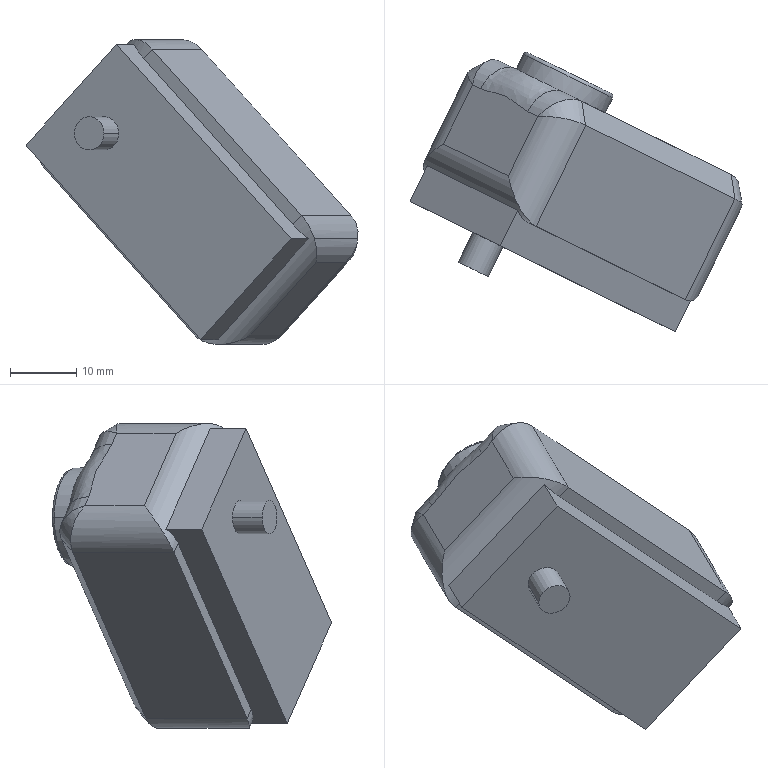Part | SolidWorks | features ICE 3, Fillet 2, Chamfer 1, Cut 1, Extrusion 1 | 1 solid | 44 faces | box 50.144 x 42.117 x 46.062 mm | volume 27040 mm3 | cylinder 19 | plane 18 | spline 5 | torus 2 | commonest cylinder face diameters 10 x11 5 x2 7.282 x2 9.108 x2 15 x2